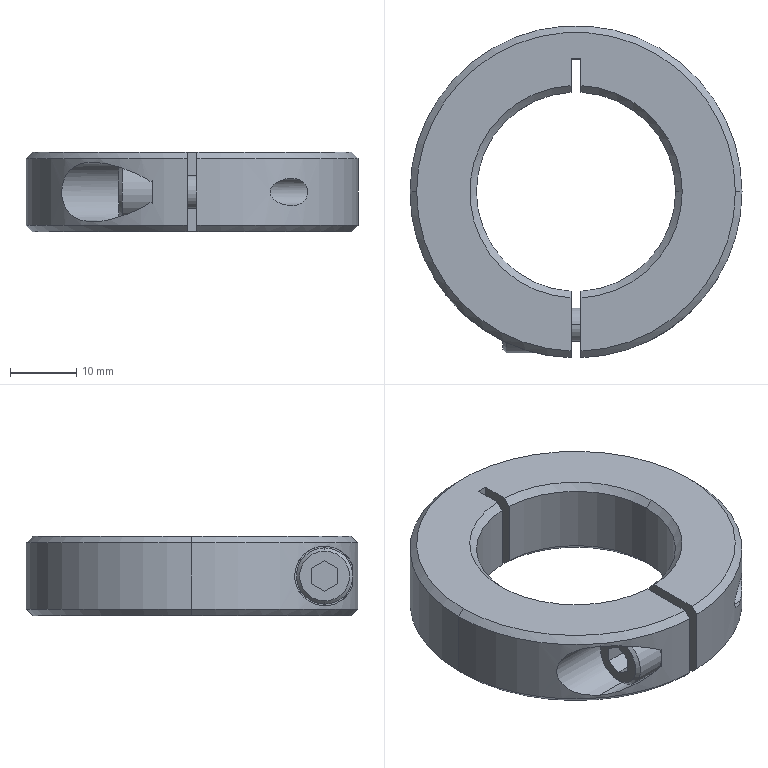Part | STEP file | FAF06-D30 | 1 solid | 51 faces | box 50 x 49.989 x 12 mm | volume 14205 mm3 | plane 18 | cylinder 17 | cone 16 | commonest cylinder face diameters 9 x3 30 x3 50 x3 4.134 x2 5 x2 5.5 x2